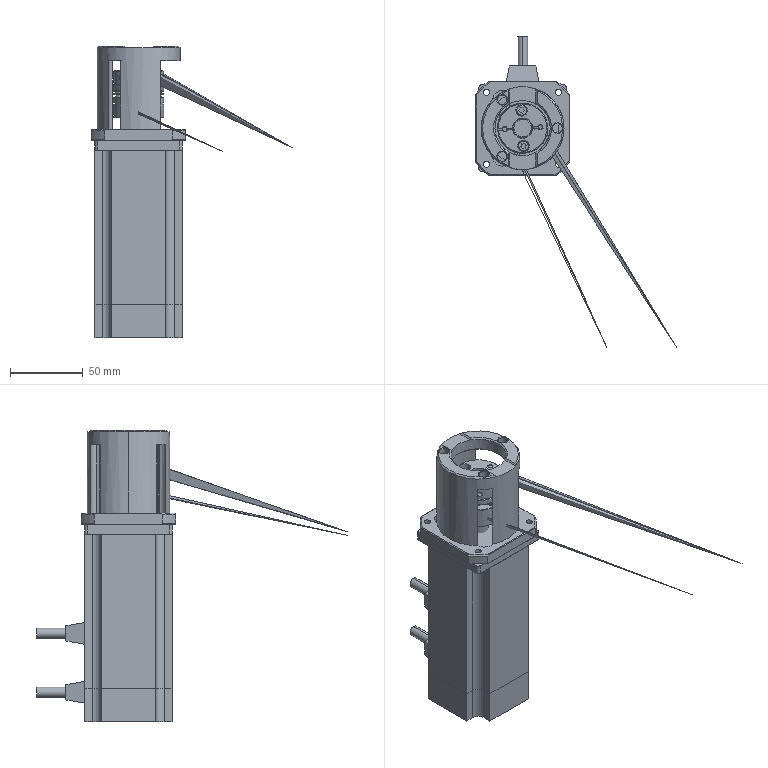Part | STEP file | Copy of 400W motor assembly (60 motor base)^K50A-1H20-S(formula driven)-L1200 right | 10 solids | 408 faces | volume 565676 mm3 | plane 175 | cylinder 166 | cone 67 | commonest cylinder face diameters 7 x32 3.3 x21 8 x19 3.1 x14 12 x12 4.2 x8